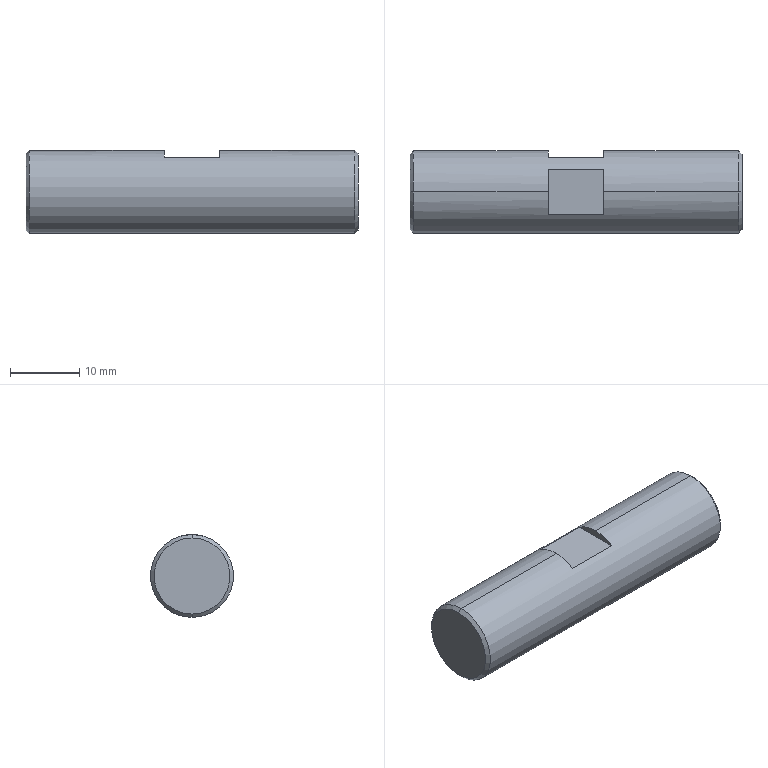Part | STEP file | 0243_004_PSFHR12-48-KFC20-G8-AG90 | 1 solid | 14 faces | box 48 x 12 x 12 mm | volume 5347 mm3 | plane 8 | cone 4 | cylinder 2 | commonest cylinder face diameters 12 x2
STEP:
#1=CARTESIAN_POINT('',(0.,0.,0.));
#2=DIRECTION('',(0.,0.,1.));
#3=DIRECTION('',(1.,0.,0.));
#4=AXIS2_PLACEMENT_3D('',#1,#2,#3);
#5=CARTESIAN_POINT('',(0.,0.,5.5));
#6=VERTEX_POINT('',#5);
#7=CARTESIAN_POINT('',(0.,0.,-5.5));
#8=VERTEX_POINT('',#7);
#9=CARTESIAN_POINT('',(0.,0.,0.));
#10=DIRECTION('',(-1.,0.,0.));
#11=DIRECTION('',(0.,0.,-1.));
#12=AXIS2_PLACEMENT_3D('',#9,#10,#11);
#13=CIRCLE('',#12,5.5);
#14=CARTESIAN_POINT('',(0.,0.,0.));
#15=DIRECTION('',(1.,0.,0.));
#16=DIRECTION('',(0.,0.,-1.));
#17=AXIS2_PLACEMENT_3D('',#14,#15,#16);
#18=CONICAL_SURFACE('',#17,5.5,0.7854);
#19=CARTESIAN_POINT('',(6.283,0.));
#20=DIRECTION('',(-1.,0.));
#21=VECTOR('',#20,1.);
#22=LINE('',#19,#21);
#23=(GEOMETRIC_REPRESENTATION_CONTEXT(2)PARAMETRIC_REPRESENTATION_CONTEXT()REPRESENTATION_CONTEXT('',''));
#24=DEFINITIONAL_REPRESENTATION('',(#22),#23);
#25=PCURVE('',#18,#24);
#26=CARTESIAN_POINT('',(0.,0.,0.));
#27=DIRECTION('',(1.,0.,0.));
#28=DIRECTION('',(0.,0.,-1.));
#29=AXIS2_PLACEMENT_3D('',#26,#27,#28);
#30=PLANE('',#29);
#31=CARTESIAN_POINT('',(5.5,0.));
#32=CARTESIAN_POINT('',(5.5,-9.526));
#33=CARTESIAN_POINT('',(-2.75,-4.763));
#34=CARTESIAN_POINT('',(-11.,0.));
#35=CARTESIAN_POINT('',(-2.75,4.763));
#36=CARTESIAN_POINT('',(5.5,9.526));
#37=CARTESIAN_POINT('',(5.5,0.));
#38=(BOUNDED_CURVE()B_SPLINE_CURVE(2,(#31,#32,#33,#34,#35,#36,#37),.UNSPECIFIED.,.T.,.F.)B_SPLINE_CURVE_WITH_KNOTS((1,2,2,2,2,1),(-2.094,0.,2.094,4.189,6.283,8.378),.UNSPECIFIED.)CURVE()GEOMETRIC_REPRESENTATION_ITEM()RATIONAL_B_SPLINE_CURVE((1.,0.5,1.,0.5,1.,0.5,1.))REPRESENTATION_ITEM(''));
#39=(GEOMETRIC_REPRESENTATION_CONTEXT(2)PARAMETRIC_REPRESENTATION_CONTEXT()REPRESENTATION_CONTEXT('',''));
#40=DEFINITIONAL_REPRESENTATION('',(#38),#39);
#41=PCURVE('',#30,#40);
#42=SURFACE_CURVE('',#13,(#25,#41),.PCURVE_S1.);
#43=EDGE_CURVE('',#6,#8,#42,.T.);
#44=ORIENTED_EDGE('',*,*,#43,.F.);
#45=CARTESIAN_POINT('',(0.5,0.,6.));
#46=VERTEX_POINT('',#45);
#47=CARTESIAN_POINT('',(0.,0.,5.5));
#48=DIRECTION('',(0.7071,0.,0.7071));
#49=VECTOR('',#48,1.);
#50=LINE('',#47,#49);
#51=CARTESIAN_POINT('',(3.142,0.));
#52=DIRECTION('',(0.,1.));
#53=VECTOR('',#52,1.);
#54=LINE('',#51,#53);
#55=(GEOMETRIC_REPRESENTATION_CONTEXT(2)PARAMETRIC_REPRESENTATION_CONTEXT()REPRESENTATION_CONTEXT('',''));
#56=DEFINITIONAL_REPRESENTATION('',(#54),#55);
#57=PCURVE('',#18,#56);
#58=CARTESIAN_POINT('',(0.,0.,0.));
#59=DIRECTION('',(1.,0.,0.));
#60=DIRECTION('',(0.,0.,-1.));
#61=AXIS2_PLACEMENT_3D('',#58,#59,#60);
#62=CONICAL_SURFACE('',#61,5.5,0.7854);
#63=CARTESIAN_POINT('',(3.142,0.));
#64=DIRECTION('',(0.,1.));
#65=VECTOR('',#64,1.);
#66=LINE('',#63,#65);
#67=(GEOMETRIC_REPRESENTATION_CONTEXT(2)PARAMETRIC_REPRESENTATION_CONTEXT()REPRESENTATION_CONTEXT('',''));
#68=DEFINITIONAL_REPRESENTATION('',(#66),#67);
#69=PCURVE('',#62,#68);
#70=SURFACE_CURVE('',#50,(#57,#69),.PCURVE_S1.);
#71=EDGE_CURVE('',#6,#46,#70,.T.);
#72=ORIENTED_EDGE('',*,*,#71,.T.);
#73=CARTESIAN_POINT('',(0.5,0.,-6.));
#74=VERTEX_POINT('',#73);
#75=CARTESIAN_POINT('',(0.5,0.,0.));
#76=DIRECTION('',(1.,0.,0.));
#77=DIRECTION('',(0.,0.,-1.));
#78=AXIS2_PLACEMENT_3D('',#75,#76,#77);
#79=CIRCLE('',#78,6.);
#80=CARTESIAN_POINT('',(0.,0.5));
#81=DIRECTION('',(1.,0.));
#82=VECTOR('',#81,1.);
#83=LINE('',#80,#82);
#84=(GEOMETRIC_REPRESENTATION_CONTEXT(2)PARAMETRIC_REPRESENTATION_CONTEXT()REPRESENTATION_CONTEXT('',''));
#85=DEFINITIONAL_REPRESENTATION('',(#83),#84);
#86=PCURVE('',#18,#85);
#87=CARTESIAN_POINT('',(-17.531,0.,0.));
#88=DIRECTION('',(-1.,0.,0.));
#89=DIRECTION('',(0.,0.,1.));
#90=AXIS2_PLACEMENT_3D('',#87,#88,#89);
#91=CYLINDRICAL_SURFACE('',#90,6.);
#92=CARTESIAN_POINT('',(3.142,-18.031));
#93=DIRECTION('',(-1.,0.));
#94=VECTOR('',#93,1.);
#95=LINE('',#92,#94);
#96=(GEOMETRIC_REPRESENTATION_CONTEXT(2)PARAMETRIC_REPRESENTATION_CONTEXT()REPRESENTATION_CONTEXT('',''));
#97=DEFINITIONAL_REPRESENTATION('',(#95),#96);
#98=PCURVE('',#91,#97);
#99=SURFACE_CURVE('',#79,(#86,#98),.PCURVE_S1.);
#100=EDGE_CURVE('',#74,#46,#99,.T.);
#101=ORIENTED_EDGE('',*,*,#100,.F.);
#102=CARTESIAN_POINT('',(0.,0.,-5.5));
#103=DIRECTION('',(0.7071,0.,-0.7071));
#104=VECTOR('',#103,1.);
#105=LINE('',#102,#104);
#106=CARTESIAN_POINT('',(0.,0.));
#107=DIRECTION('',(0.,1.));
#108=VECTOR('',#107,1.);
#109=LINE('',#106,#108);
#110=(GEOMETRIC_REPRESENTATION_CONTEXT(2)PARAMETRIC_REPRESENTATION_CONTEXT()REPRESENTATION_CONTEXT('',''));
#111=DEFINITIONAL_REPRESENTATION('',(#109),#110);
#112=PCURVE('',#18,#111);
#113=CARTESIAN_POINT('',(6.283,0.));
#114=DIRECTION('',(0.,1.));
#115=VECTOR('',#114,1.);
#116=LINE('',#113,#115);
#117=(GEOMETRIC_REPRESENTATION_CONTEXT(2)PARAMETRIC_REPRESENTATION_CONTEXT()REPRESENTATION_CONTEXT('',''));
#118=DEFINITIONAL_REPRESENTATION('',(#116),#117);
#119=PCURVE('',#62,#118);
#120=SURFACE_CURVE('',#105,(#112,#119),.PCURVE_S1.);
#121=EDGE_CURVE('',#8,#74,#120,.T.);
#122=ORIENTED_EDGE('',*,*,#121,.F.);
#123=EDGE_LOOP('',(#44,#72,#101,#122));
#124=FACE_BOUND('',#123,.T.);
#125=ADVANCED_FACE('',(#124),#18,.T.);
#126=CARTESIAN_POINT('',(48.,0.,-5.5));
#127=VERTEX_POINT('',#126);
#128=CARTESIAN_POINT('',(48.,0.,5.5));
#129=VERTEX_POINT('',#128);
#130=CARTESIAN_POINT('',(48.,0.,0.));
#131=DIRECTION('',(1.,0.,0.));
#132=DIRECTION('',(0.,0.,1.));
#133=AXIS2_PLACEMENT_3D('',#130,#131,#132);
#134=CIRCLE('',#133,5.5);
#135=CARTESIAN_POINT('',(47.5,0.,0.));
#136=DIRECTION('',(-1.,0.,0.));
#137=DIRECTION('',(0.,0.,1.));
#138=AXIS2_PLACEMENT_3D('',#135,#136,#137);
#139=CONICAL_SURFACE('',#138,6.,0.7854);
#140=CARTESIAN_POINT('',(6.283,-0.5));
#141=DIRECTION('',(-1.,0.));
#142=VECTOR('',#141,1.);
#143=LINE('',#140,#142);
#144=(GEOMETRIC_REPRESENTATION_CONTEXT(2)PARAMETRIC_REPRESENTATION_CONTEXT()REPRESENTATION_CONTEXT('',''));
#145=DEFINITIONAL_REPRESENTATION('',(#143),#144);
#146=PCURVE('',#139,#145);
#147=CARTESIAN_POINT('',(48.,6.,0.));
#148=DIRECTION('',(-1.,0.,0.));
#149=DIRECTION('',(0.,0.,1.));
#150=AXIS2_PLACEMENT_3D('',#147,#148,#149);
#151=PLANE('',#150);
#152=CARTESIAN_POINT('',(5.5,-6.));
#153=CARTESIAN_POINT('',(5.5,-15.526));
#154=CARTESIAN_POINT('',(-2.75,-10.763));
#155=CARTESIAN_POINT('',(-11.,-6.));
#156=CARTESIAN_POINT('',(-2.75,-1.237));
#157=CARTESIAN_POINT('',(5.5,3.526));
#158=CARTESIAN_POINT('',(5.5,-6.));
#159=(BOUNDED_CURVE()B_SPLINE_CURVE(2,(#152,#153,#154,#155,#156,#157,#158),.UNSPECIFIED.,.T.,.F.)B_SPLINE_CURVE_WITH_KNOTS((1,2,2,2,2,1),(-2.094,0.,2.094,4.189,6.283,8.378),.UNSPECIFIED.)CURVE()GEOMETRIC_REPRESENTATION_ITEM()RATIONAL_B_SPLINE_CURVE((1.,0.5,1.,0.5,1.,0.5,1.))REPRESENTATION_ITEM(''));
#160=(GEOMETRIC_REPRESENTATION_CONTEXT(2)PARAMETRIC_REPRESENTATION_CONTEXT()REPRESENTATION_CONTEXT('',''));
#161=DEFINITIONAL_REPRESENTATION('',(#159),#160);
#162=PCURVE('',#151,#161);
#163=SURFACE_CURVE('',#134,(#146,#162),.PCURVE_S1.);
#164=EDGE_CURVE('',#127,#129,#163,.T.);
#165=ORIENTED_EDGE('',*,*,#164,.F.);
#166=CARTESIAN_POINT('',(47.5,0.,-6.));
#167=VERTEX_POINT('',#166);
#168=CARTESIAN_POINT('',(47.5,0.,-6.));
#169=DIRECTION('',(-0.7071,0.,-0.7071));
#170=VECTOR('',#169,1.);
#171=LINE('',#168,#170);
#172=CARTESIAN_POINT('',(3.142,0.));
#173=DIRECTION('',(0.,1.));
#174=VECTOR('',#173,1.);
#175=LINE('',#172,#174);
#176=(GEOMETRIC_REPRESENTATION_CONTEXT(2)PARAMETRIC_REPRESENTATION_CONTEXT()REPRESENTATION_CONTEXT('',''));
#177=DEFINITIONAL_REPRESENTATION('',(#175),#176);
#178=PCURVE('',#139,#177);
#179=CARTESIAN_POINT('',(47.5,0.,0.));
#180=DIRECTION('',(-1.,0.,0.));
#181=DIRECTION('',(0.,0.,1.));
#182=AXIS2_PLACEMENT_3D('',#179,#180,#181);
#183=CONICAL_SURFACE('',#182,6.,0.7854);
#184=CARTESIAN_POINT('',(3.142,0.));
#185=DIRECTION('',(0.,1.));
#186=VECTOR('',#185,1.);
#187=LINE('',#184,#186);
#188=(GEOMETRIC_REPRESENTATION_CONTEXT(2)PARAMETRIC_REPRESENTATION_CONTEXT()REPRESENTATION_CONTEXT('',''));
#189=DEFINITIONAL_REPRESENTATION('',(#187),#188);
#190=PCURVE('',#183,#189);
#191=SURFACE_CURVE('',#171,(#178,#190),.PCURVE_S1.);
#192=EDGE_CURVE('',#127,#167,#191,.T.);
#193=ORIENTED_EDGE('',*,*,#192,.T.);
#194=CARTESIAN_POINT('',(47.5,0.,6.));
#195=VERTEX_POINT('',#194);
#196=CARTESIAN_POINT('',(47.5,0.,0.));
#197=DIRECTION('',(-1.,0.,0.));
#198=DIRECTION('',(0.,0.,1.));
#199=AXIS2_PLACEMENT_3D('',#196,#197,#198);
#200=CIRCLE('',#199,6.);
#201=CARTESIAN_POINT('',(0.,0.));
#202=DIRECTION('',(1.,0.));
#203=VECTOR('',#202,1.);
#204=LINE('',#201,#203);
#205=(GEOMETRIC_REPRESENTATION_CONTEXT(2)PARAMETRIC_REPRESENTATION_CONTEXT()REPRESENTATION_CONTEXT('',''));
#206=DEFINITIONAL_REPRESENTATION('',(#204),#205);
#207=PCURVE('',#139,#206);
#208=CARTESIAN_POINT('',(0.,-65.031));
#209=DIRECTION('',(1.,0.));
#210=VECTOR('',#209,1.);
#211=LINE('',#208,#210);
#212=(GEOMETRIC_REPRESENTATION_CONTEXT(2)PARAMETRIC_REPRESENTATION_CONTEXT()REPRESENTATION_CONTEXT('',''));
#213=DEFINITIONAL_REPRESENTATION('',(#211),#212);
#214=PCURVE('',#91,#213);
#215=SURFACE_CURVE('',#200,(#207,#214),.PCURVE_S1.);
#216=EDGE_CURVE('',#195,#167,#215,.T.);
#217=ORIENTED_EDGE('',*,*,#216,.F.);
#218=CARTESIAN_POINT('',(47.5,0.,6.));
#219=DIRECTION('',(-0.7071,0.,0.7071));
#220=VECTOR('',#219,1.);
#221=LINE('',#218,#220);
#222=CARTESIAN_POINT('',(0.,0.));
#223=DIRECTION('',(0.,1.));
#224=VECTOR('',#223,1.);
#225=LINE('',#222,#224);
#226=(GEOMETRIC_REPRESENTATION_CONTEXT(2)PARAMETRIC_REPRESENTATION_CONTEXT()REPRESENTATION_CONTEXT('',''));
#227=DEFINITIONAL_REPRESENTATION('',(#225),#226);
#228=PCURVE('',#139,#227);
#229=CARTESIAN_POINT('',(6.283,0.));
#230=DIRECTION('',(0.,1.));
#231=VECTOR('',#230,1.);
#232=LINE('',#229,#231);
#233=(GEOMETRIC_REPRESENTATION_CONTEXT(2)PARAMETRIC_REPRESENTATION_CONTEXT()REPRESENTATION_CONTEXT('',''));
#234=DEFINITIONAL_REPRESENTATION('',(#232),#233);
#235=PCURVE('',#183,#234);
#236=SURFACE_CURVE('',#221,(#228,#235),.PCURVE_S1.);
#237=EDGE_CURVE('',#129,#195,#236,.T.);
#238=ORIENTED_EDGE('',*,*,#237,.F.);
#239=EDGE_LOOP('',(#165,#193,#217,#238));
#240=FACE_BOUND('',#239,.T.);
#241=ADVANCED_FACE('',(#240),#139,.T.);
#242=CARTESIAN_POINT('',(28.,5.,-3.317));
#243=VERTEX_POINT('',#242);
#244=CARTESIAN_POINT('',(28.,5.,3.317));
#245=VERTEX_POINT('',#244);
#246=CARTESIAN_POINT('',(28.,0.,0.));
#247=DIRECTION('',(1.,0.,0.));
#248=DIRECTION('',(0.,1.,0.));
#249=AXIS2_PLACEMENT_3D('',#246,#247,#248);
#250=CIRCLE('',#249,6.);
#251=CARTESIAN_POINT('',(7.854,-45.531));
#252=DIRECTION('',(-1.,0.));
#253=VECTOR('',#252,1.);
#254=LINE('',#251,#253);
#255=(GEOMETRIC_REPRESENTATION_CONTEXT(2)PARAMETRIC_REPRESENTATION_CONTEXT()REPRESENTATION_CONTEXT('',''));
#256=DEFINITIONAL_REPRESENTATION('',(#254),#255);
#257=PCURVE('',#91,#256);
#258=CARTESIAN_POINT('',(28.,6.,-6.));
#259=DIRECTION('',(1.,0.,0.));
#260=DIRECTION('',(0.,1.,0.));
#261=AXIS2_PLACEMENT_3D('',#258,#259,#260);
#262=PLANE('',#261);
#263=CARTESIAN_POINT('',(-6.,6.));
#264=DIRECTION('',(1.,0.));
#265=AXIS2_PLACEMENT_2D('',#263,#264);
#266=CIRCLE('',#265,6.);
#267=(GEOMETRIC_REPRESENTATION_CONTEXT(2)PARAMETRIC_REPRESENTATION_CONTEXT()REPRESENTATION_CONTEXT('',''));
#268=DEFINITIONAL_REPRESENTATION('',(#266),#267);
#269=PCURVE('',#262,#268);
#270=SURFACE_CURVE('',#250,(#257,#269),.PCURVE_S1.);
#271=EDGE_CURVE('',#243,#245,#270,.T.);
#272=ORIENTED_EDGE('',*,*,#271,.T.);
#273=CARTESIAN_POINT('',(20.,5.,3.317));
#274=VERTEX_POINT('',#273);
#275=CARTESIAN_POINT('',(-17.531,5.,3.317));
#276=DIRECTION('',(-1.,0.,0.));
#277=VECTOR('',#276,1.);
#278=LINE('',#275,#277);
#279=CARTESIAN_POINT('',(0.9851,0.));
#280=DIRECTION('',(0.,1.));
#281=VECTOR('',#280,1.);
#282=LINE('',#279,#281);
#283=(GEOMETRIC_REPRESENTATION_CONTEXT(2)PARAMETRIC_REPRESENTATION_CONTEXT()REPRESENTATION_CONTEXT('',''));
#284=DEFINITIONAL_REPRESENTATION('',(#282),#283);
#285=PCURVE('',#91,#284);
#286=CARTESIAN_POINT('',(20.,5.,-6.));
#287=DIRECTION('',(0.,-1.,0.));
#288=DIRECTION('',(0.,0.,-1.));
#289=AXIS2_PLACEMENT_3D('',#286,#287,#288);
#290=PLANE('',#289);
#291=CARTESIAN_POINT('',(-9.317,-37.531));
#292=DIRECTION('',(0.,-1.));
#293=VECTOR('',#292,1.);
#294=LINE('',#291,#293);
#295=(GEOMETRIC_REPRESENTATION_CONTEXT(2)PARAMETRIC_REPRESENTATION_CONTEXT()REPRESENTATION_CONTEXT('',''));
#296=DEFINITIONAL_REPRESENTATION('',(#294),#295);
#297=PCURVE('',#290,#296);
#298=SURFACE_CURVE('',#278,(#285,#297),.PCURVE_S1.);
#299=EDGE_CURVE('',#245,#274,#298,.T.);
#300=ORIENTED_EDGE('',*,*,#299,.T.);
#301=CARTESIAN_POINT('',(20.,5.,-3.317));
#302=VERTEX_POINT('',#301);
#303=CARTESIAN_POINT('',(20.,0.,0.));
#304=DIRECTION('',(-1.,0.,0.));
#305=DIRECTION('',(0.,0.,1.));
#306=AXIS2_PLACEMENT_3D('',#303,#304,#305);
#307=CIRCLE('',#306,6.);
#308=CARTESIAN_POINT('',(0.,-37.531));
#309=DIRECTION('',(1.,0.));
#310=VECTOR('',#309,1.);
#311=LINE('',#308,#310);
#312=(GEOMETRIC_REPRESENTATION_CONTEXT(2)PARAMETRIC_REPRESENTATION_CONTEXT()REPRESENTATION_CONTEXT('',''));
#313=DEFINITIONAL_REPRESENTATION('',(#311),#312);
#314=PCURVE('',#91,#313);
#315=CARTESIAN_POINT('',(20.,6.,-6.));
#316=DIRECTION('',(-1.,0.,0.));
#317=DIRECTION('',(0.,0.,1.));
#318=AXIS2_PLACEMENT_3D('',#315,#316,#317);
#319=PLANE('',#318);
#320=CARTESIAN_POINT('',(6.,-6.));
#321=DIRECTION('',(1.,0.));
#322=AXIS2_PLACEMENT_2D('',#320,#321);
#323=CIRCLE('',#322,6.);
#324=(GEOMETRIC_REPRESENTATION_CONTEXT(2)PARAMETRIC_REPRESENTATION_CONTEXT()REPRESENTATION_CONTEXT('',''));
#325=DEFINITIONAL_REPRESENTATION('',(#323),#324);
#326=PCURVE('',#319,#325);
#327=SURFACE_CURVE('',#307,(#314,#326),.PCURVE_S1.);
#328=EDGE_CURVE('',#274,#302,#327,.T.);
#329=ORIENTED_EDGE('',*,*,#328,.T.);
#330=CARTESIAN_POINT('',(-17.531,5.,-3.317));
#331=DIRECTION('',(1.,0.,0.));
#332=VECTOR('',#331,1.);
#333=LINE('',#330,#332);
#334=CARTESIAN_POINT('',(2.156,0.));
#335=DIRECTION('',(0.,-1.));
#336=VECTOR('',#335,1.);
#337=LINE('',#334,#336);
#338=(GEOMETRIC_REPRESENTATION_CONTEXT(2)PARAMETRIC_REPRESENTATION_CONTEXT()REPRESENTATION_CONTEXT('',''));
#339=DEFINITIONAL_REPRESENTATION('',(#337),#338);
#340=PCURVE('',#91,#339);
#341=CARTESIAN_POINT('',(-2.683,-37.531));
#342=DIRECTION('',(0.,1.));
#343=VECTOR('',#342,1.);
#344=LINE('',#341,#343);
#345=(GEOMETRIC_REPRESENTATION_CONTEXT(2)PARAMETRIC_REPRESENTATION_CONTEXT()REPRESENTATION_CONTEXT('',''));
#346=DEFINITIONAL_REPRESENTATION('',(#344),#345);
#347=PCURVE('',#290,#346);
#348=SURFACE_CURVE('',#333,(#340,#347),.PCURVE_S1.);
#349=EDGE_CURVE('',#302,#243,#348,.T.);
#350=ORIENTED_EDGE('',*,*,#349,.T.);
#351=EDGE_LOOP('',(#272,#300,#329,#350));
#352=FACE_BOUND('',#351,.T.);
#353=ORIENTED_EDGE('',*,*,#216,.T.);
#354=CARTESIAN_POINT('',(-17.531,0.,-6.));
#355=DIRECTION('',(-1.,0.,0.));
#356=VECTOR('',#355,1.);
#357=LINE('',#354,#356);
#358=CARTESIAN_POINT('',(3.142,0.));
#359=DIRECTION('',(0.,1.));
#360=VECTOR('',#359,1.);
#361=LINE('',#358,#360);
#362=(GEOMETRIC_REPRESENTATION_CONTEXT(2)PARAMETRIC_REPRESENTATION_CONTEXT()REPRESENTATION_CONTEXT('',''));
#363=DEFINITIONAL_REPRESENTATION('',(#361),#362);
#364=PCURVE('',#91,#363);
#365=CARTESIAN_POINT('',(-17.531,0.,0.));
#366=DIRECTION('',(-1.,0.,0.));
#367=DIRECTION('',(0.,0.,1.));
#368=AXIS2_PLACEMENT_3D('',#365,#366,#367);
#369=CYLINDRICAL_SURFACE('',#368,6.);
#370=CARTESIAN_POINT('',(3.142,0.));
#371=DIRECTION('',(0.,1.));
#372=VECTOR('',#371,1.);
#373=LINE('',#370,#372);
#374=(GEOMETRIC_REPRESENTATION_CONTEXT(2)PARAMETRIC_REPRESENTATION_CONTEXT()REPRESENTATION_CONTEXT('',''));
#375=DEFINITIONAL_REPRESENTATION('',(#373),#374);
#376=PCURVE('',#369,#375);
#377=SURFACE_CURVE('',#357,(#364,#376),.PCURVE_S1.);
#378=EDGE_CURVE('',#167,#74,#377,.T.);
#379=ORIENTED_EDGE('',*,*,#378,.T.);
#380=ORIENTED_EDGE('',*,*,#100,.T.);
#381=CARTESIAN_POINT('',(20.,0.,6.));
#382=VERTEX_POINT('',#381);
#383=CARTESIAN_POINT('',(-17.531,0.,6.));
#384=DIRECTION('',(-1.,0.,0.));
#385=VECTOR('',#384,1.);
#386=LINE('',#383,#385);
#387=CARTESIAN_POINT('',(0.,0.));
#388=DIRECTION('',(0.,1.));
#389=VECTOR('',#388,1.);
#390=LINE('',#387,#389);
#391=(GEOMETRIC_REPRESENTATION_CONTEXT(2)PARAMETRIC_REPRESENTATION_CONTEXT()REPRESENTATION_CONTEXT('',''));
#392=DEFINITIONAL_REPRESENTATION('',(#390),#391);
#393=PCURVE('',#91,#392);
#394=CARTESIAN_POINT('',(6.283,0.));
#395=DIRECTION('',(0.,1.));
#396=VECTOR('',#395,1.);
#397=LINE('',#394,#396);
#398=(GEOMETRIC_REPRESENTATION_CONTEXT(2)PARAMETRIC_REPRESENTATION_CONTEXT()REPRESENTATION_CONTEXT('',''));
#399=DEFINITIONAL_REPRESENTATION('',(#397),#398);
#400=PCURVE('',#369,#399);
#401=SURFACE_CURVE('',#386,(#393,#400),.PCURVE_S1.);
#402=EDGE_CURVE('',#382,#46,#401,.T.);
#403=ORIENTED_EDGE('',*,*,#402,.F.);
#404=CARTESIAN_POINT('',(20.,3.317,5.));
#405=VERTEX_POINT('',#404);
#406=CARTESIAN_POINT('',(20.,0.,0.));
#407=DIRECTION('',(-1.,0.,0.));
#408=DIRECTION('',(0.,0.,1.));
#409=AXIS2_PLACEMENT_3D('',#406,#407,#408);
#410=CIRCLE('',#409,6.);
#411=CARTESIAN_POINT('',(0.,-37.531));
#412=DIRECTION('',(1.,0.));
#413=VECTOR('',#412,1.);
#414=LINE('',#411,#413);
#415=(GEOMETRIC_REPRESENTATION_CONTEXT(2)PARAMETRIC_REPRESENTATION_CONTEXT()REPRESENTATION_CONTEXT('',''));
#416=DEFINITIONAL_REPRESENTATION('',(#414),#415);
#417=PCURVE('',#91,#416);
#418=CARTESIAN_POINT('',(20.,6.,6.));
#419=DIRECTION('',(-1.,0.,0.));
#420=DIRECTION('',(0.,0.,1.));
#421=AXIS2_PLACEMENT_3D('',#418,#419,#420);
#422=PLANE('',#421);
#423=CARTESIAN_POINT('',(-6.,-6.));
#424=DIRECTION('',(1.,0.));
#425=AXIS2_PLACEMENT_2D('',#423,#424);
#426=CIRCLE('',#425,6.);
#427=(GEOMETRIC_REPRESENTATION_CONTEXT(2)PARAMETRIC_REPRESENTATION_CONTEXT()REPRESENTATION_CONTEXT('',''));
#428=DEFINITIONAL_REPRESENTATION('',(#426),#427);
#429=PCURVE('',#422,#428);
#430=SURFACE_CURVE('',#410,(#417,#429),.PCURVE_S1.);
#431=EDGE_CURVE('',#382,#405,#430,.T.);
#432=ORIENTED_EDGE('',*,*,#431,.T.);
#433=CARTESIAN_POINT('',(28.,3.317,5.));
#434=VERTEX_POINT('',#433);
#435=CARTESIAN_POINT('',(-17.531,3.317,5.));
#436=DIRECTION('',(1.,0.,0.));
#437=VECTOR('',#436,1.);
#438=LINE('',#435,#437);
#439=CARTESIAN_POINT('',(0.5857,0.));
#440=DIRECTION('',(0.,-1.));
#441=VECTOR('',#440,1.);
#442=LINE('',#439,#441);
#443=(GEOMETRIC_REPRESENTATION_CONTEXT(2)PARAMETRIC_REPRESENTATION_CONTEXT()REPRESENTATION_CONTEXT('',''));
#444=DEFINITIONAL_REPRESENTATION('',(#442),#443);
#445=PCURVE('',#91,#444);
#446=CARTESIAN_POINT('',(20.,6.,5.));
#447=DIRECTION('',(0.,0.,-1.));
#448=DIRECTION('',(0.,1.,0.));
#449=AXIS2_PLACEMENT_3D('',#446,#447,#448);
#450=PLANE('',#449);
#451=CARTESIAN_POINT('',(-2.683,-37.531));
#452=DIRECTION('',(0.,1.));
#453=VECTOR('',#452,1.);
#454=LINE('',#451,#453);
#455=(GEOMETRIC_REPRESENTATION_CONTEXT(2)PARAMETRIC_REPRESENTATION_CONTEXT()REPRESENTATION_CONTEXT('',''));
#456=DEFINITIONAL_REPRESENTATION('',(#454),#455);
#457=PCURVE('',#450,#456);
#458=SURFACE_CURVE('',#438,(#445,#457),.PCURVE_S1.);
#459=EDGE_CURVE('',#405,#434,#458,.T.);
#460=ORIENTED_EDGE('',*,*,#459,.T.);
#461=CARTESIAN_POINT('',(28.,0.,6.));
#462=VERTEX_POINT('',#461);
#463=CARTESIAN_POINT('',(28.,0.,0.));
#464=DIRECTION('',(1.,0.,0.));
#465=DIRECTION('',(0.,0.,-1.));
#466=AXIS2_PLACEMENT_3D('',#463,#464,#465);
#467=CIRCLE('',#466,6.);
#468=CARTESIAN_POINT('',(3.142,-45.531));
#469=DIRECTION('',(-1.,0.));
#470=VECTOR('',#469,1.);
#471=LINE('',#468,#470);
#472=(GEOMETRIC_REPRESENTATION_CONTEXT(2)PARAMETRIC_REPRESENTATION_CONTEXT()REPRESENTATION_CONTEXT('',''));
#473=DEFINITIONAL_REPRESENTATION('',(#471),#472);
#474=PCURVE('',#91,#473);
#475=CARTESIAN_POINT('',(28.,6.,6.));
#476=DIRECTION('',(1.,0.,0.));
#477=DIRECTION('',(0.,0.,-1.));
#478=AXIS2_PLACEMENT_3D('',#475,#476,#477);
#479=PLANE('',#478);
#480=CARTESIAN_POINT('',(6.,-6.));
#481=DIRECTION('',(1.,0.));
#482=AXIS2_PLACEMENT_2D('',#480,#481);
#483=CIRCLE('',#482,6.);
#484=(GEOMETRIC_REPRESENTATION_CONTEXT(2)PARAMETRIC_REPRESENTATION_CONTEXT()REPRESENTATION_CONTEXT('',''));
#485=DEFINITIONAL_REPRESENTATION('',(#483),#484);
#486=PCURVE('',#479,#485);
#487=SURFACE_CURVE('',#467,(#474,#486),.PCURVE_S1.);
#488=EDGE_CURVE('',#434,#462,#487,.T.);
#489=ORIENTED_EDGE('',*,*,#488,.T.);
#490=CARTESIAN_POINT('',(-17.531,0.,6.));
#491=DIRECTION('',(-1.,0.,0.));
#492=VECTOR('',#491,1.);
#493=LINE('',#490,#492);
#494=CARTESIAN_POINT('',(0.,0.));
#495=DIRECTION('',(0.,1.));
#496=VECTOR('',#495,1.);
#497=LINE('',#494,#496);
#498=(GEOMETRIC_REPRESENTATION_CONTEXT(2)PARAMETRIC_REPRESENTATION_CONTEXT()REPRESENTATION_CONTEXT('',''));
#499=DEFINITIONAL_REPRESENTATION('',(#497),#498);
#500=PCURVE('',#91,#499);
#501=CARTESIAN_POINT('',(6.283,0.));
#502=DIRECTION('',(0.,1.));
#503=VECTOR('',#502,1.);
#504=LINE('',#501,#503);
#505=(GEOMETRIC_REPRESENTATION_CONTEXT(2)PARAMETRIC_REPRESENTATION_CONTEXT()REPRESENTATION_CONTEXT('',''));
#506=DEFINITIONAL_REPRESENTATION('',(#504),#505);
#507=PCURVE('',#369,#506);
#508=SURFACE_CURVE('',#493,(#500,#507),.PCURVE_S1.);
#509=EDGE_CURVE('',#195,#462,#508,.T.);
#510=ORIENTED_EDGE('',*,*,#509,.F.);
#511=EDGE_LOOP('',(#353,#379,#380,#403,#432,#460,#489,#510));
#512=FACE_BOUND('',#511,.T.);
#513=ADVANCED_FACE('',(#352,#512),#91,.T.);
#514=CARTESIAN_POINT('',(0.,0.,0.));
#515=DIRECTION('',(-1.,0.,0.));
#516=DIRECTION('',(0.,0.,-1.));
#517=AXIS2_PLACEMENT_3D('',#514,#515,#516);
#518=CIRCLE('',#517,5.5);
#519=CARTESIAN_POINT('',(5.5,0.));
#520=CARTESIAN_POINT('',(5.5,-9.526));
#521=CARTESIAN_POINT('',(-2.75,-4.763));
#522=CARTESIAN_POINT('',(-11.,0.));
#523=CARTESIAN_POINT('',(-2.75,4.763));
#524=CARTESIAN_POINT('',(5.5,9.526));
#525=CARTESIAN_POINT('',(5.5,0.));
#526=(BOUNDED_CURVE()B_SPLINE_CURVE(2,(#519,#520,#521,#522,#523,#524,#525),.UNSPECIFIED.,.T.,.F.)B_SPLINE_CURVE_WITH_KNOTS((1,2,2,2,2,1),(-2.094,0.,2.094,4.189,6.283,8.378),.UNSPECIFIED.)CURVE()GEOMETRIC_REPRESENTATION_ITEM()RATIONAL_B_SPLINE_CURVE((1.,0.5,1.,0.5,1.,0.5,1.))REPRESENTATION_ITEM(''));
#527=(GEOMETRIC_REPRESENTATION_CONTEXT(2)PARAMETRIC_REPRESENTATION_CONTEXT()REPRESENTATION_CONTEXT('',''));
#528=DEFINITIONAL_REPRESENTATION('',(#526),#527);
#529=PCURVE('',#30,#528);
#530=CARTESIAN_POINT('',(6.283,0.));
#531=DIRECTION('',(-1.,0.));
#532=VECTOR('',#531,1.);
#533=LINE('',#530,#532);
#534=(GEOMETRIC_REPRESENTATION_CONTEXT(2)PARAMETRIC_REPRESENTATION_CONTEXT()REPRESENTATION_CONTEXT('',''));
#535=DEFINITIONAL_REPRESENTATION('',(#533),#534);
#536=PCURVE('',#62,#535);
#537=SURFACE_CURVE('',#518,(#529,#536),.PCURVE_S1.);
#538=EDGE_CURVE('',#8,#6,#537,.T.);
#539=ORIENTED_EDGE('',*,*,#538,.T.);
#540=ORIENTED_EDGE('',*,*,#43,.T.);
#541=EDGE_LOOP('',(#539,#540));
#542=FACE_BOUND('',#541,.T.);
#543=ADVANCED_FACE('',(#542),#30,.F.);
#544=ORIENTED_EDGE('',*,*,#378,.F.);
#545=CARTESIAN_POINT('',(47.5,0.,0.));
#546=DIRECTION('',(-1.,0.,0.));
#547=DIRECTION('',(0.,0.,1.));
#548=AXIS2_PLACEMENT_3D('',#545,#546,#547);
#549=CIRCLE('',#548,6.);
#550=CARTESIAN_POINT('',(0.,-65.031));
#551=DIRECTION('',(1.,0.));
#552=VECTOR('',#551,1.);
#553=LINE('',#550,#552);
#554=(GEOMETRIC_REPRESENTATION_CONTEXT(2)PARAMETRIC_REPRESENTATION_CONTEXT()REPRESENTATION_CONTEXT('',''));
#555=DEFINITIONAL_REPRESENTATION('',(#553),#554);
#556=PCURVE('',#369,#555);
#557=CARTESIAN_POINT('',(0.,0.));
#558=DIRECTION('',(1.,0.));
#559=VECTOR('',#558,1.);
#560=LINE('',#557,#559);
#561=(GEOMETRIC_REPRESENTATION_CONTEXT(2)PARAMETRIC_REPRESENTATION_CONTEXT()REPRESENTATION_CONTEXT('',''));
#562=DEFINITIONAL_REPRESENTATION('',(#560),#561);
#563=PCURVE('',#183,#562);
#564=SURFACE_CURVE('',#549,(#556,#563),.PCURVE_S1.);
#565=EDGE_CURVE('',#167,#195,#564,.T.);
#566=ORIENTED_EDGE('',*,*,#565,.T.);
#567=ORIENTED_EDGE('',*,*,#509,.T.);
#568=CARTESIAN_POINT('',(28.,-3.317,5.));
#569=VERTEX_POINT('',#568);
#570=CARTESIAN_POINT('',(28.,0.,0.));
#571=DIRECTION('',(1.,0.,0.));
#572=DIRECTION('',(0.,0.,-1.));
#573=AXIS2_PLACEMENT_3D('',#570,#571,#572);
#574=CIRCLE('',#573,6.);
#575=CARTESIAN_POINT('',(9.425,-45.531));
#576=DIRECTION('',(-1.,0.));
#577=VECTOR('',#576,1.);
#578=LINE('',#575,#577);
#579=(GEOMETRIC_REPRESENTATION_CONTEXT(2)PARAMETRIC_REPRESENTATION_CONTEXT()REPRESENTATION_CONTEXT('',''));
#580=DEFINITIONAL_REPRESENTATION('',(#578),#579);
#581=PCURVE('',#369,#580);
#582=CARTESIAN_POINT('',(6.,-6.));
#583=DIRECTION('',(1.,0.));
#584=AXIS2_PLACEMENT_2D('',#582,#583);
#585=CIRCLE('',#584,6.);
#586=(GEOMETRIC_REPRESENTATION_CONTEXT(2)PARAMETRIC_REPRESENTATION_CONTEXT()REPRESENTATION_CONTEXT('',''));
#587=DEFINITIONAL_REPRESENTATION('',(#585),#586);
#588=PCURVE('',#479,#587);
#589=SURFACE_CURVE('',#574,(#581,#588),.PCURVE_S1.);
#590=EDGE_CURVE('',#462,#569,#589,.T.);
#591=ORIENTED_EDGE('',*,*,#590,.T.);
#592=CARTESIAN_POINT('',(20.,-3.317,5.));
#593=VERTEX_POINT('',#592);
#594=CARTESIAN_POINT('',(-17.531,-3.317,5.));
#595=DIRECTION('',(-1.,0.,0.));
#596=VECTOR('',#595,1.);
#597=LINE('',#594,#596);
#598=CARTESIAN_POINT('',(5.697,0.));
#599=DIRECTION('',(0.,1.));
#600=VECTOR('',#599,1.);
#601=LINE('',#598,#600);
#602=(GEOMETRIC_REPRESENTATION_CONTEXT(2)PARAMETRIC_REPRESENTATION_CONTEXT()REPRESENTATION_CONTEXT('',''));
#603=DEFINITIONAL_REPRESENTATION('',(#601),#602);
#604=PCURVE('',#369,#603);
#605=CARTESIAN_POINT('',(-9.317,-37.531));
#606=DIRECTION('',(0.,-1.));
#607=VECTOR('',#606,1.);
#608=LINE('',#605,#607);
#609=(GEOMETRIC_REPRESENTATION_CONTEXT(2)PARAMETRIC_REPRESENTATION_CONTEXT()REPRESENTATION_CONTEXT('',''));
#610=DEFINITIONAL_REPRESENTATION('',(#608),#609);
#611=PCURVE('',#450,#610);
#612=SURFACE_CURVE('',#597,(#604,#611),.PCURVE_S1.);
#613=EDGE_CURVE('',#569,#593,#612,.T.);
#614=ORIENTED_EDGE('',*,*,#613,.T.);
#615=CARTESIAN_POINT('',(20.,0.,0.));
#616=DIRECTION('',(-1.,0.,0.));
#617=DIRECTION('',(0.,0.,1.));
#618=AXIS2_PLACEMENT_3D('',#615,#616,#617);
#619=CIRCLE('',#618,6.);
#620=CARTESIAN_POINT('',(0.,-37.531));
#621=DIRECTION('',(1.,0.));
#622=VECTOR('',#621,1.);
#623=LINE('',#620,#622);
#624=(GEOMETRIC_REPRESENTATION_CONTEXT(2)PARAMETRIC_REPRESENTATION_CONTEXT()REPRESENTATION_CONTEXT('',''));
#625=DEFINITIONAL_REPRESENTATION('',(#623),#624);
#626=PCURVE('',#369,#625);
#627=CARTESIAN_POINT('',(-6.,-6.));
#628=DIRECTION('',(1.,0.));
#629=AXIS2_PLACEMENT_2D('',#627,#628);
#630=CIRCLE('',#629,6.);
#631=(GEOMETRIC_REPRESENTATION_CONTEXT(2)PARAMETRIC_REPRESENTATION_CONTEXT()REPRESENTATION_CONTEXT('',''));
#632=DEFINITIONAL_REPRESENTATION('',(#630),#631);
#633=PCURVE('',#422,#632);
#634=SURFACE_CURVE('',#619,(#626,#633),.PCURVE_S1.);
#635=EDGE_CURVE('',#593,#382,#634,.T.);
#636=ORIENTED_EDGE('',*,*,#635,.T.);
#637=ORIENTED_EDGE('',*,*,#402,.T.);
#638=CARTESIAN_POINT('',(0.5,0.,0.));
#639=DIRECTION('',(1.,0.,0.));
#640=DIRECTION('',(0.,0.,-1.));
#641=AXIS2_PLACEMENT_3D('',#638,#639,#640);
#642=CIRCLE('',#641,6.);
#643=CARTESIAN_POINT('',(9.425,-18.031));
#644=DIRECTION('',(-1.,0.));
#645=VECTOR('',#644,1.);
#646=LINE('',#643,#645);
#647=(GEOMETRIC_REPRESENTATION_CONTEXT(2)PARAMETRIC_REPRESENTATION_CONTEXT()REPRESENTATION_CONTEXT('',''));
#648=DEFINITIONAL_REPRESENTATION('',(#646),#647);
#649=PCURVE('',#369,#648);
#650=CARTESIAN_POINT('',(0.,0.5));
#651=DIRECTION('',(1.,0.));
#652=VECTOR('',#651,1.);
#653=LINE('',#650,#652);
#654=(GEOMETRIC_REPRESENTATION_CONTEXT(2)PARAMETRIC_REPRESENTATION_CONTEXT()REPRESENTATION_CONTEXT('',''));
#655=DEFINITIONAL_REPRESENTATION('',(#653),#654);
#656=PCURVE('',#62,#655);
#657=SURFACE_CURVE('',#642,(#649,#656),.PCURVE_S1.);
#658=EDGE_CURVE('',#46,#74,#657,.T.);
#659=ORIENTED_EDGE('',*,*,#658,.T.);
#660=EDGE_LOOP('',(#544,#566,#567,#591,#614,#636,#637,#659));
#661=FACE_BOUND('',#660,.T.);
#662=ADVANCED_FACE('',(#661),#369,.T.);
#663=CARTESIAN_POINT('',(48.,0.,0.));
#664=DIRECTION('',(1.,0.,0.));
#665=DIRECTION('',(0.,0.,1.));
#666=AXIS2_PLACEMENT_3D('',#663,#664,#665);
#667=CIRCLE('',#666,5.5);
#668=CARTESIAN_POINT('',(5.5,-6.));
#669=CARTESIAN_POINT('',(5.5,-15.526));
#670=CARTESIAN_POINT('',(-2.75,-10.763));
#671=CARTESIAN_POINT('',(-11.,-6.));
#672=CARTESIAN_POINT('',(-2.75,-1.237));
#673=CARTESIAN_POINT('',(5.5,3.526));
#674=CARTESIAN_POINT('',(5.5,-6.));
#675=(BOUNDED_CURVE()B_SPLINE_CURVE(2,(#668,#669,#670,#671,#672,#673,#674),.UNSPECIFIED.,.T.,.F.)B_SPLINE_CURVE_WITH_KNOTS((1,2,2,2,2,1),(-2.094,0.,2.094,4.189,6.283,8.378),.UNSPECIFIED.)CURVE()GEOMETRIC_REPRESENTATION_ITEM()RATIONAL_B_SPLINE_CURVE((1.,0.5,1.,0.5,1.,0.5,1.))REPRESENTATION_ITEM(''));
#676=(GEOMETRIC_REPRESENTATION_CONTEXT(2)PARAMETRIC_REPRESENTATION_CONTEXT()REPRESENTATION_CONTEXT('',''));
#677=DEFINITIONAL_REPRESENTATION('',(#675),#676);
#678=PCURVE('',#151,#677);
#679=CARTESIAN_POINT('',(6.283,-0.5));
#680=DIRECTION('',(-1.,0.));
#681=VECTOR('',#680,1.);
#682=LINE('',#679,#681);
#683=(GEOMETRIC_REPRESENTATION_CONTEXT(2)PARAMETRIC_REPRESENTATION_CONTEXT()REPRESENTATION_CONTEXT('',''));
#684=DEFINITIONAL_REPRESENTATION('',(#682),#683);
#685=PCURVE('',#183,#684);
#686=SURFACE_CURVE('',#667,(#678,#685),.PCURVE_S1.);
#687=EDGE_CURVE('',#129,#127,#686,.T.);
#688=ORIENTED_EDGE('',*,*,#687,.T.);
#689=ORIENTED_EDGE('',*,*,#164,.T.);
#690=EDGE_LOOP('',(#688,#689));
#691=FACE_BOUND('',#690,.T.);
#692=ADVANCED_FACE('',(#691),#151,.F.);
#693=CARTESIAN_POINT('',(20.,5.,-6.));
#694=DIRECTION('',(0.,0.,1.));
#695=VECTOR('',#694,1.);
#696=LINE('',#693,#695);
#697=CARTESIAN_POINT('',(0.,-1.));
#698=DIRECTION('',(1.,0.));
#699=VECTOR('',#698,1.);
#700=LINE('',#697,#699);
#701=(GEOMETRIC_REPRESENTATION_CONTEXT(2)PARAMETRIC_REPRESENTATION_CONTEXT()REPRESENTATION_CONTEXT('',''));
#702=DEFINITIONAL_REPRESENTATION('',(#700),#701);
#703=PCURVE('',#319,#702);
#704=CARTESIAN_POINT('',(0.,0.));
#705=DIRECTION('',(-1.,0.));
#706=VECTOR('',#705,1.);
#707=LINE('',#704,#706);
#708=(GEOMETRIC_REPRESENTATION_CONTEXT(2)PARAMETRIC_REPRESENTATION_CONTEXT()REPRESENTATION_CONTEXT('',''));
#709=DEFINITIONAL_REPRESENTATION('',(#707),#708);
#710=PCURVE('',#290,#709);
#711=SURFACE_CURVE('',#696,(#703,#710),.PCURVE_S1.);
#712=EDGE_CURVE('',#302,#274,#711,.T.);
#713=ORIENTED_EDGE('',*,*,#712,.F.);
#714=ORIENTED_EDGE('',*,*,#328,.F.);
#715=EDGE_LOOP('',(#713,#714));
#716=FACE_BOUND('',#715,.T.);
#717=ADVANCED_FACE('',(#716),#319,.F.);
#718=ORIENTED_EDGE('',*,*,#271,.F.);
#719=CARTESIAN_POINT('',(28.,5.,-6.));
#720=DIRECTION('',(0.,0.,1.));
#721=VECTOR('',#720,1.);
#722=LINE('',#719,#721);
#723=CARTESIAN_POINT('',(-1.,0.));
#724=DIRECTION('',(0.,1.));
#725=VECTOR('',#724,1.);
#726=LINE('',#723,#725);
#727=(GEOMETRIC_REPRESENTATION_CONTEXT(2)PARAMETRIC_REPRESENTATION_CONTEXT()REPRESENTATION_CONTEXT('',''));
#728=DEFINITIONAL_REPRESENTATION('',(#726),#727);
#729=PCURVE('',#262,#728);
#730=CARTESIAN_POINT('',(0.,8.));
#731=DIRECTION('',(-1.,0.));
#732=VECTOR('',#731,1.);
#733=LINE('',#730,#732);
#734=(GEOMETRIC_REPRESENTATION_CONTEXT(2)PARAMETRIC_REPRESENTATION_CONTEXT()REPRESENTATION_CONTEXT('',''));
#735=DEFINITIONAL_REPRESENTATION('',(#733),#734);
#736=PCURVE('',#290,#735);
#737=SURFACE_CURVE('',#722,(#729,#736),.PCURVE_S1.);
#738=EDGE_CURVE('',#243,#245,#737,.T.);
#739=ORIENTED_EDGE('',*,*,#738,.T.);
#740=EDGE_LOOP('',(#718,#739));
#741=FACE_BOUND('',#740,.T.);
#742=ADVANCED_FACE('',(#741),#262,.F.);
#743=ORIENTED_EDGE('',*,*,#738,.F.);
#744=ORIENTED_EDGE('',*,*,#349,.F.);
#745=ORIENTED_EDGE('',*,*,#712,.T.);
#746=ORIENTED_EDGE('',*,*,#299,.F.);
#747=EDGE_LOOP('',(#743,#744,#745,#746));
#748=FACE_BOUND('',#747,.T.);
#749=ADVANCED_FACE('',(#748),#290,.F.);
#750=ORIENTED_EDGE('',*,*,#635,.F.);
#751=CARTESIAN_POINT('',(20.,6.,5.));
#752=DIRECTION('',(0.,-1.,0.));
#753=VECTOR('',#752,1.);
#754=LINE('',#751,#753);
#755=CARTESIAN_POINT('',(-1.,0.));
#756=DIRECTION('',(0.,-1.));
#757=VECTOR('',#756,1.);
#758=LINE('',#755,#757);
#759=(GEOMETRIC_REPRESENTATION_CONTEXT(2)PARAMETRIC_REPRESENTATION_CONTEXT()REPRESENTATION_CONTEXT('',''));
#760=DEFINITIONAL_REPRESENTATION('',(#758),#759);
#761=PCURVE('',#422,#760);
#762=CARTESIAN_POINT('',(0.,0.));
#763=DIRECTION('',(-1.,0.));
#764=VECTOR('',#763,1.);
#765=LINE('',#762,#764);
#766=(GEOMETRIC_REPRESENTATION_CONTEXT(2)PARAMETRIC_REPRESENTATION_CONTEXT()REPRESENTATION_CONTEXT('',''));
#767=DEFINITIONAL_REPRESENTATION('',(#765),#766);
#768=PCURVE('',#450,#767);
#769=SURFACE_CURVE('',#754,(#761,#768),.PCURVE_S1.);
#770=EDGE_CURVE('',#405,#593,#769,.T.);
#771=ORIENTED_EDGE('',*,*,#770,.F.);
#772=ORIENTED_EDGE('',*,*,#431,.F.);
#773=EDGE_LOOP('',(#750,#771,#772));
#774=FACE_BOUND('',#773,.T.);
#775=ADVANCED_FACE('',(#774),#422,.F.);
#776=CARTESIAN_POINT('',(28.,6.,5.));
#777=DIRECTION('',(0.,-1.,0.));
#778=VECTOR('',#777,1.);
#779=LINE('',#776,#778);
#780=CARTESIAN_POINT('',(1.,0.));
#781=DIRECTION('',(0.,-1.));
#782=VECTOR('',#781,1.);
#783=LINE('',#780,#782);
#784=(GEOMETRIC_REPRESENTATION_CONTEXT(2)PARAMETRIC_REPRESENTATION_CONTEXT()REPRESENTATION_CONTEXT('',''));
#785=DEFINITIONAL_REPRESENTATION('',(#783),#784);
#786=PCURVE('',#479,#785);
#787=CARTESIAN_POINT('',(0.,8.));
#788=DIRECTION('',(-1.,0.));
#789=VECTOR('',#788,1.);
#790=LINE('',#787,#789);
#791=(GEOMETRIC_REPRESENTATION_CONTEXT(2)PARAMETRIC_REPRESENTATION_CONTEXT()REPRESENTATION_CONTEXT('',''));
#792=DEFINITIONAL_REPRESENTATION('',(#790),#791);
#793=PCURVE('',#450,#792);
#794=SURFACE_CURVE('',#779,(#786,#793),.PCURVE_S1.);
#795=EDGE_CURVE('',#434,#569,#794,.T.);
#796=ORIENTED_EDGE('',*,*,#795,.T.);
#797=ORIENTED_EDGE('',*,*,#590,.F.);
#798=ORIENTED_EDGE('',*,*,#488,.F.);
#799=EDGE_LOOP('',(#796,#797,#798));
#800=FACE_BOUND('',#799,.T.);
#801=ADVANCED_FACE('',(#800),#479,.F.);
#802=ORIENTED_EDGE('',*,*,#795,.F.);
#803=ORIENTED_EDGE('',*,*,#459,.F.);
#804=ORIENTED_EDGE('',*,*,#770,.T.);
#805=ORIENTED_EDGE('',*,*,#613,.F.);
#806=EDGE_LOOP('',(#802,#803,#804,#805));
#807=FACE_BOUND('',#806,.T.);
#808=ADVANCED_FACE('',(#807),#450,.F.);
#809=ORIENTED_EDGE('',*,*,#192,.F.);
#810=ORIENTED_EDGE('',*,*,#687,.F.);
#811=ORIENTED_EDGE('',*,*,#237,.T.);
#812=ORIENTED_EDGE('',*,*,#565,.F.);
#813=EDGE_LOOP('',(#809,#810,#811,#812));
#814=FACE_BOUND('',#813,.T.);
#815=ADVANCED_FACE('',(#814),#183,.T.);
#816=ORIENTED_EDGE('',*,*,#71,.F.);
#817=ORIENTED_EDGE('',*,*,#538,.F.);
#818=ORIENTED_EDGE('',*,*,#121,.T.);
#819=ORIENTED_EDGE('',*,*,#658,.F.);
#820=EDGE_LOOP('',(#816,#817,#818,#819));
#821=FACE_BOUND('',#820,.T.);
#822=ADVANCED_FACE('',(#821),#62,.T.);
#823=CLOSED_SHELL('',(#125,#241,#513,#543,#662,#692,#717,#742,#749,#775,#801,#808,#815,#822));
#824=MANIFOLD_SOLID_BREP('',#823);
#825=(LENGTH_UNIT()NAMED_UNIT(*)SI_UNIT(.MILLI.,.METRE.));
#826=UNCERTAINTY_MEASURE_WITH_UNIT(LENGTH_MEASURE(0.0000001),#825,'','');
#827=(NAMED_UNIT(*)PLANE_ANGLE_UNIT()SI_UNIT($,.RADIAN.));
#828=(NAMED_UNIT(*)SI_UNIT($,.STERADIAN.)SOLID_ANGLE_UNIT());
#829=(GEOMETRIC_REPRESENTATION_CONTEXT(3)GLOBAL_UNCERTAINTY_ASSIGNED_CONTEXT((#826))GLOBAL_UNIT_ASSIGNED_CONTEXT((#825,#827,#828))REPRESENTATION_CONTEXT('',''));
#830=ADVANCED_BREP_SHAPE_REPRESENTATION('',(#4,#824),#829);